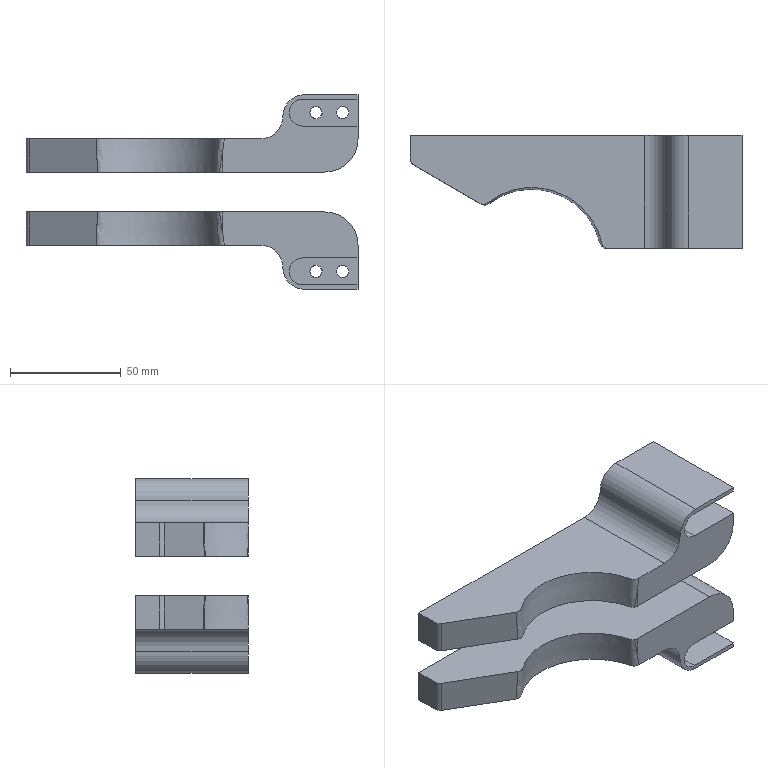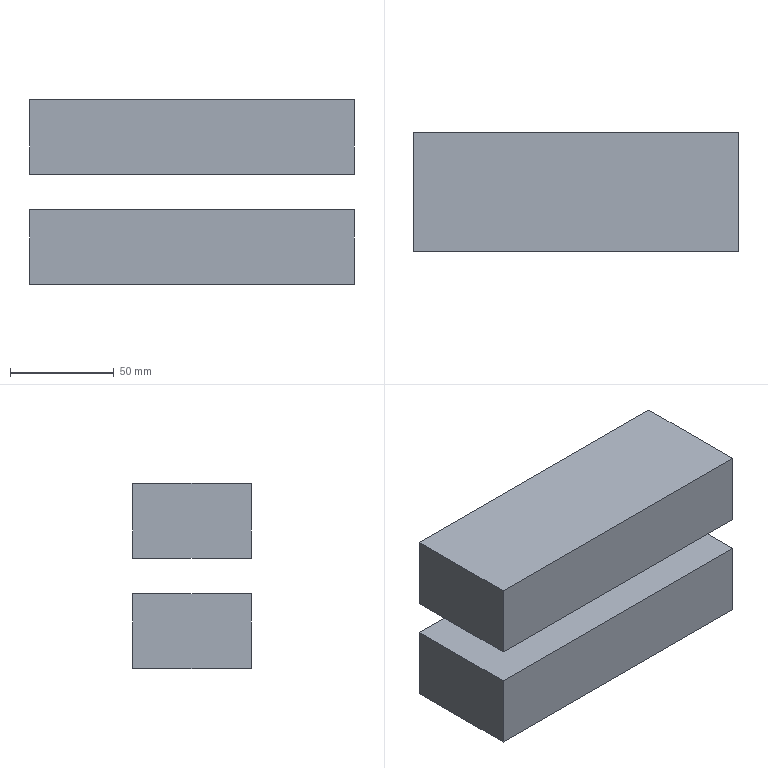CAM job | NX | 3-axis milling, drilling | part box 150 x 51 x 88 mm | stock box 156 x 57 x 89 mm
Tools:
number,name,description,diameter,corner_radius,flute_length,length,flutes
1,D63,Milling Tool-5 Parameters,63.0,0.0,50.0,75.0,2
7,D6A45,Milling Tool-5 Parameters,6.0,0.0,50.0,75.0,2
15,5.5ZT,Drilling Tool,5.5,0.0,35.0,50.0,2
12,D12C,Milling Tool-5 Parameters,12.0,0.0,50.0,75.0,2
11,D12JING,Milling Tool-5 Parameters,11.99,0.0,50.0,75.0,2
8,R4,Milling Tool-5 Parameters,8.0,4.0,50.0,75.0,2
Operations:
program,operation,operation_type,tool,method,geometry_group,spindle_rpm,surface_speed,feed_per_tooth,feed_cut,feed_plunge,cut_length_mm,path_length_mm,cut_time_min,machine_time_min
1,FLOOR_WALL,VolumeBased25DMillingOperation,D63,METHOD,A,6500.0,1286.0,0.1154,1500.0,100.0,230.999,284.999,0.154,0.1594
1,DRILLING,Operation,D6A45,METHOD,A,5000.0,94.0,0.025,250.0,0.0,8.0,91.369,0.032,0.0403
1,DRILLING_COPY,Operation,5.5ZT,METHOD,A,2000.0,34.0,0.03,120.0,0.0,113.305,301.979,0.9442,0.9631
1,ADAPTIVE_MILLING,CavityMilling,D12C,METHOD,A,9500.0,358.0,0.1579,3000.0,1000.0,15019.362,15665.86,5.014,5.079
1,CAVITY_MILL,CavityMilling,D12C,METHOD,A,9500.0,358.0,0.1316,2500.0,1000.0,10077.933,10627.672,4.536,4.591
1,ZLEVEL_PROFILE_COPY_COPY_COPY_1_COPY_COPY_COPY,ZLevelMilling,D12JING,METHOD,A,9500.0,358.0,0.0632,1200.0,1000.0,2411.45,2581.446,2.014,2.031
1,ZLEVEL_PROFILE,ZLevelMilling,D12JING,METHOD,A,9500.0,179.0,0.0868,1650.0,100.0,1032.055,1112.195,0.6255,0.6335
1,PLANAR_MILL,PlanarMilling,D6A45,METHOD,A,9500.0,179.0,0.0658,1250.0,100.0,222.815,282.815,0.1783,0.1843
1,FIXED_CONTOUR,SurfaceContour,R4,METHOD,A,9500.0,119.0,0.1579,3000.0,100.0,14854.959,14946.159,4.952,4.961
1,FIXED_CONTOUR_1,SurfaceContour,R4,METHOD,A,9500.0,119.0,0.1579,3000.0,100.0,1129.463,1263.863,0.3765,0.3899
2,FLOOR_WALL_COPY,VolumeBased25DMillingOperation,D63,METHOD,B,6500.0,1286.0,0.1154,1500.0,100.0,230.999,284.999,0.154,0.1594
2,DRILLING_COPY_1,Operation,D6A45,METHOD,B,5000.0,94.0,0.025,250.0,0.0,8.0,91.369,0.032,0.0403
2,DRILLING_COPY_COPY,Operation,5.5ZT,METHOD,B,2000.0,34.0,0.03,120.0,0.0,113.305,301.979,0.9442,0.9631
2,ADAPTIVE_MILLING_COPY,CavityMilling,D12C,METHOD,B,9500.0,358.0,0.1579,3000.0,1000.0,14921.345,15304.715,4.98,5.018
2,CAVITY_MILL_COPY,CavityMilling,D12C,METHOD,B,9500.0,358.0,0.1316,2500.0,1000.0,10036.181,10464.682,4.509,4.552
2,ZLEVEL_PROFILE_COPY_COPY_COPY_1_COPY_COPY_COPY_COPY,ZLevelMilling,D12JING,METHOD,B,9500.0,358.0,0.0632,1200.0,1000.0,2410.051,2579.762,2.013,2.03
2,ZLEVEL_PROFILE_COPY,ZLevelMilling,D12JING,METHOD,B,9500.0,179.0,0.0868,1650.0,100.0,1032.055,1112.195,0.6255,0.6335
2,FIXED_CONTOUR_COPY,SurfaceContour,R4,METHOD,B,9500.0,119.0,0.1579,3000.0,100.0,14854.959,14946.159,4.952,4.961
2,FIXED_CONTOUR_1_COPY,SurfaceContour,R4,METHOD,B,9500.0,119.0,0.1579,3000.0,100.0,1129.463,1263.863,0.3765,0.3899